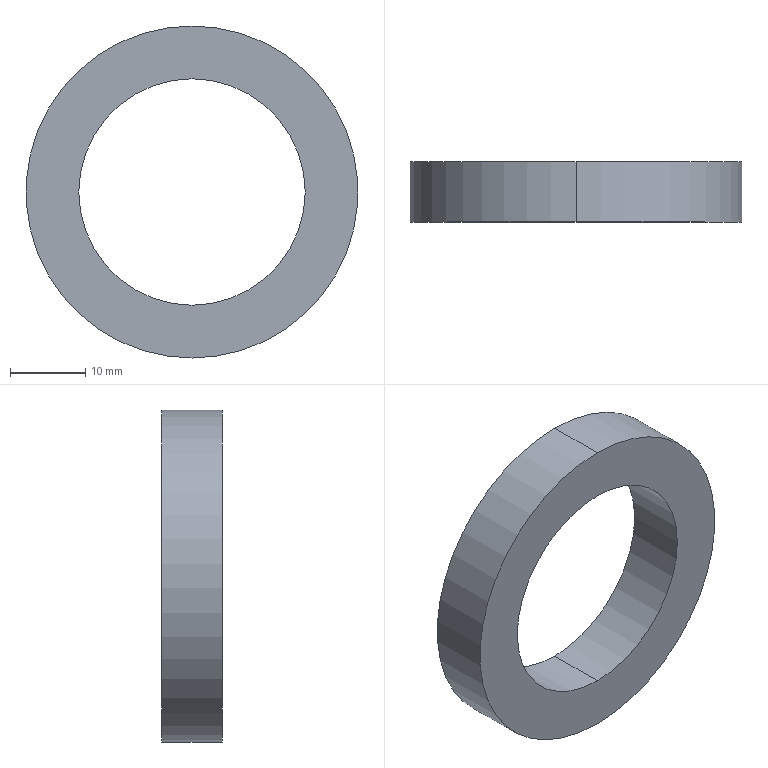Part | SolidWorks | features BaseBody 1 | 1 solid | 6 faces | box 44 x 8 x 44 mm | volume 6509 mm3 | cylinder 4 | plane 2 | commonest cylinder face diameters 30 x2 44 x2
STEP:
#1=CARTESIAN_POINT('',(0.,8.,15.));
#2=VERTEX_POINT('',#1);
#3=CARTESIAN_POINT('',(0.,8.,-15.));
#4=VERTEX_POINT('',#3);
#5=CARTESIAN_POINT('',(0.,8.,0.));
#6=DIRECTION('',(0.,-1.,0.));
#7=DIRECTION('',(0.,0.,-1.));
#8=AXIS2_PLACEMENT_3D('',#5,#6,#7);
#9=CIRCLE('',#8,15.);
#10=EDGE_CURVE('',#2,#4,#9,.T.);
#11=ORIENTED_EDGE('',*,*,#10,.F.);
#12=CARTESIAN_POINT('',(0.,0.,15.));
#13=VERTEX_POINT('',#12);
#14=CARTESIAN_POINT('',(0.,8.,15.));
#15=DIRECTION('',(0.,-1.,0.));
#16=VECTOR('',#15,1000.);
#17=LINE('',#14,#16);
#18=EDGE_CURVE('',#2,#13,#17,.T.);
#19=ORIENTED_EDGE('',*,*,#18,.T.);
#20=CARTESIAN_POINT('',(0.,0.,-15.));
#21=VERTEX_POINT('',#20);
#22=CARTESIAN_POINT('',(0.,0.,0.));
#23=DIRECTION('',(0.,1.,0.));
#24=DIRECTION('',(0.,0.,-1.));
#25=AXIS2_PLACEMENT_3D('',#22,#23,#24);
#26=CIRCLE('',#25,15.);
#27=EDGE_CURVE('',#21,#13,#26,.T.);
#28=ORIENTED_EDGE('',*,*,#27,.F.);
#29=CARTESIAN_POINT('',(0.,8.,-15.));
#30=DIRECTION('',(0.,-1.,0.));
#31=VECTOR('',#30,1000.);
#32=LINE('',#29,#31);
#33=EDGE_CURVE('',#4,#21,#32,.T.);
#34=ORIENTED_EDGE('',*,*,#33,.F.);
#35=EDGE_LOOP('',(#11,#19,#28,#34));
#36=FACE_OUTER_BOUND('',#35,.T.);
#37=CARTESIAN_POINT('',(0.,8.,0.));
#38=DIRECTION('',(0.,-1.,0.));
#39=DIRECTION('',(0.,0.,-1.));
#40=AXIS2_PLACEMENT_3D('',#37,#38,#39);
#41=CYLINDRICAL_SURFACE('',#40,15.);
#42=ADVANCED_FACE('',(#36),#41,.F.);
#43=CARTESIAN_POINT('',(0.,8.,22.));
#44=VERTEX_POINT('',#43);
#45=CARTESIAN_POINT('',(0.,8.,-22.));
#46=VERTEX_POINT('',#45);
#47=CARTESIAN_POINT('',(0.,8.,0.));
#48=DIRECTION('',(0.,1.,0.));
#49=DIRECTION('',(0.,0.,-1.));
#50=AXIS2_PLACEMENT_3D('',#47,#48,#49);
#51=CIRCLE('',#50,22.);
#52=EDGE_CURVE('',#44,#46,#51,.T.);
#53=ORIENTED_EDGE('',*,*,#52,.F.);
#54=CARTESIAN_POINT('',(0.,0.,22.));
#55=VERTEX_POINT('',#54);
#56=CARTESIAN_POINT('',(0.,8.,22.));
#57=DIRECTION('',(0.,-1.,0.));
#58=VECTOR('',#57,1000.);
#59=LINE('',#56,#58);
#60=EDGE_CURVE('',#44,#55,#59,.T.);
#61=ORIENTED_EDGE('',*,*,#60,.T.);
#62=CARTESIAN_POINT('',(0.,0.,-22.));
#63=VERTEX_POINT('',#62);
#64=CARTESIAN_POINT('',(0.,0.,0.));
#65=DIRECTION('',(0.,1.,0.));
#66=DIRECTION('',(0.,0.,-1.));
#67=AXIS2_PLACEMENT_3D('',#64,#65,#66);
#68=CIRCLE('',#67,22.);
#69=EDGE_CURVE('',#55,#63,#68,.T.);
#70=ORIENTED_EDGE('',*,*,#69,.T.);
#71=CARTESIAN_POINT('',(0.,8.,-22.));
#72=DIRECTION('',(0.,-1.,0.));
#73=VECTOR('',#72,1000.);
#74=LINE('',#71,#73);
#75=EDGE_CURVE('',#46,#63,#74,.T.);
#76=ORIENTED_EDGE('',*,*,#75,.F.);
#77=EDGE_LOOP('',(#53,#61,#70,#76));
#78=FACE_OUTER_BOUND('',#77,.T.);
#79=CARTESIAN_POINT('',(0.,8.,0.));
#80=DIRECTION('',(0.,-1.,0.));
#81=DIRECTION('',(0.,0.,-1.));
#82=AXIS2_PLACEMENT_3D('',#79,#80,#81);
#83=CYLINDRICAL_SURFACE('',#82,22.);
#84=ADVANCED_FACE('',(#78),#83,.T.);
#85=CARTESIAN_POINT('',(0.,8.,0.));
#86=DIRECTION('',(0.,-1.,0.));
#87=DIRECTION('',(0.,0.,-1.));
#88=AXIS2_PLACEMENT_3D('',#85,#86,#87);
#89=CIRCLE('',#88,15.);
#90=EDGE_CURVE('',#4,#2,#89,.T.);
#91=ORIENTED_EDGE('',*,*,#90,.T.);
#92=ORIENTED_EDGE('',*,*,#10,.T.);
#93=EDGE_LOOP('',(#91,#92));
#94=FACE_BOUND('',#93,.T.);
#95=CARTESIAN_POINT('',(0.,8.,0.));
#96=DIRECTION('',(0.,1.,0.));
#97=DIRECTION('',(0.,0.,-1.));
#98=AXIS2_PLACEMENT_3D('',#95,#96,#97);
#99=CIRCLE('',#98,22.);
#100=EDGE_CURVE('',#46,#44,#99,.T.);
#101=ORIENTED_EDGE('',*,*,#100,.T.);
#102=ORIENTED_EDGE('',*,*,#52,.T.);
#103=EDGE_LOOP('',(#101,#102));
#104=FACE_OUTER_BOUND('',#103,.T.);
#105=CARTESIAN_POINT('',(0.,8.,0.));
#106=DIRECTION('',(0.,1.,0.));
#107=DIRECTION('',(0.,0.,1.));
#108=AXIS2_PLACEMENT_3D('',#105,#106,#107);
#109=PLANE('',#108);
#110=ADVANCED_FACE('',(#94,#104),#109,.T.);
#111=ORIENTED_EDGE('',*,*,#18,.F.);
#112=ORIENTED_EDGE('',*,*,#90,.F.);
#113=ORIENTED_EDGE('',*,*,#33,.T.);
#114=CARTESIAN_POINT('',(0.,0.,0.));
#115=DIRECTION('',(0.,1.,0.));
#116=DIRECTION('',(0.,0.,-1.));
#117=AXIS2_PLACEMENT_3D('',#114,#115,#116);
#118=CIRCLE('',#117,15.);
#119=EDGE_CURVE('',#13,#21,#118,.T.);
#120=ORIENTED_EDGE('',*,*,#119,.F.);
#121=EDGE_LOOP('',(#111,#112,#113,#120));
#122=FACE_OUTER_BOUND('',#121,.T.);
#123=CARTESIAN_POINT('',(0.,8.,0.));
#124=DIRECTION('',(0.,-1.,0.));
#125=DIRECTION('',(0.,0.,-1.));
#126=AXIS2_PLACEMENT_3D('',#123,#124,#125);
#127=CYLINDRICAL_SURFACE('',#126,15.);
#128=ADVANCED_FACE('',(#122),#127,.F.);
#129=ORIENTED_EDGE('',*,*,#60,.F.);
#130=ORIENTED_EDGE('',*,*,#100,.F.);
#131=ORIENTED_EDGE('',*,*,#75,.T.);
#132=CARTESIAN_POINT('',(0.,0.,0.));
#133=DIRECTION('',(0.,1.,0.));
#134=DIRECTION('',(0.,0.,-1.));
#135=AXIS2_PLACEMENT_3D('',#132,#133,#134);
#136=CIRCLE('',#135,22.);
#137=EDGE_CURVE('',#63,#55,#136,.T.);
#138=ORIENTED_EDGE('',*,*,#137,.T.);
#139=EDGE_LOOP('',(#129,#130,#131,#138));
#140=FACE_OUTER_BOUND('',#139,.T.);
#141=CARTESIAN_POINT('',(0.,8.,0.));
#142=DIRECTION('',(0.,-1.,0.));
#143=DIRECTION('',(0.,0.,-1.));
#144=AXIS2_PLACEMENT_3D('',#141,#142,#143);
#145=CYLINDRICAL_SURFACE('',#144,22.);
#146=ADVANCED_FACE('',(#140),#145,.T.);
#147=ORIENTED_EDGE('',*,*,#27,.T.);
#148=ORIENTED_EDGE('',*,*,#119,.T.);
#149=EDGE_LOOP('',(#147,#148));
#150=FACE_BOUND('',#149,.T.);
#151=ORIENTED_EDGE('',*,*,#137,.F.);
#152=ORIENTED_EDGE('',*,*,#69,.F.);
#153=EDGE_LOOP('',(#151,#152));
#154=FACE_OUTER_BOUND('',#153,.T.);
#155=CARTESIAN_POINT('',(0.,0.,0.));
#156=DIRECTION('',(0.,1.,0.));
#157=DIRECTION('',(0.,0.,1.));
#158=AXIS2_PLACEMENT_3D('',#155,#156,#157);
#159=PLANE('',#158);
#160=ADVANCED_FACE('',(#150,#154),#159,.F.);
#161=CLOSED_SHELL('',(#42,#84,#110,#128,#146,#160));
#162=MANIFOLD_SOLID_BREP('',#161);
#163=CARTESIAN_POINT('',(0.,0.,0.));
#164=DIRECTION('',(0.,0.,1.));
#165=DIRECTION('',(1.,0.,0.));
#166=AXIS2_PLACEMENT_3D('',#163,#164,#165);
#167=(LENGTH_UNIT()NAMED_UNIT(*)SI_UNIT(.MILLI.,.METRE.));
#168=UNCERTAINTY_MEASURE_WITH_UNIT(LENGTH_MEASURE(0.00001),#167,'','');
#169=(NAMED_UNIT(*)PLANE_ANGLE_UNIT()SI_UNIT($,.RADIAN.));
#170=(NAMED_UNIT(*)SI_UNIT($,.STERADIAN.)SOLID_ANGLE_UNIT());
#171=(GEOMETRIC_REPRESENTATION_CONTEXT(3)GLOBAL_UNCERTAINTY_ASSIGNED_CONTEXT((#168))GLOBAL_UNIT_ASSIGNED_CONTEXT((#167,#169,#170))REPRESENTATION_CONTEXT('',''));
#172=ADVANCED_BREP_SHAPE_REPRESENTATION('',(#162,#166),#171);